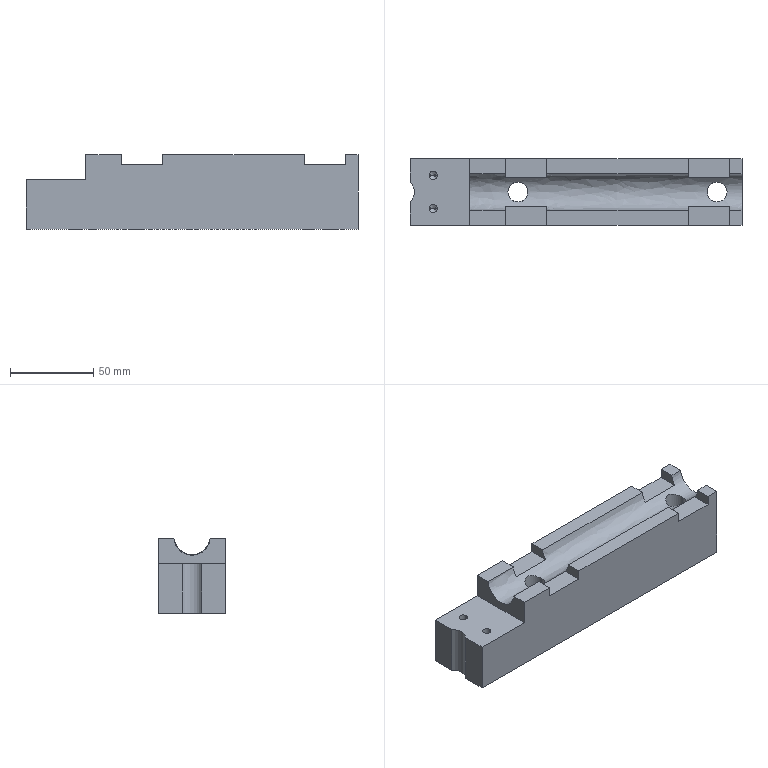Part | 1 solid | 72 faces | volume 292155 mm3 | plane 26 | cylinder 25 | cone 20 | spline 1 | commonest cylinder face diameters 7 x12 5 x8 12 x4 15.5 x1